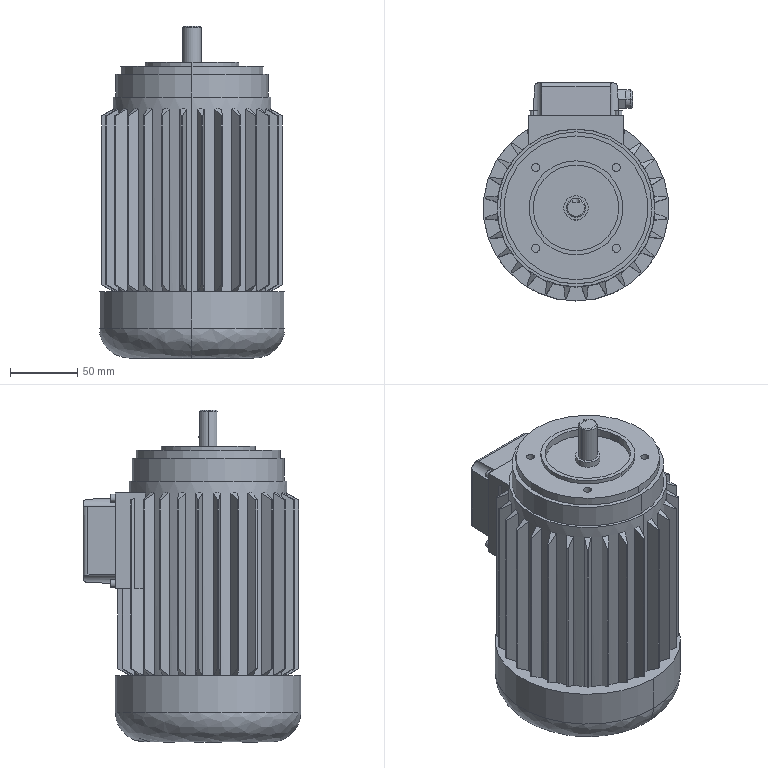Part | STEP file | Motor_P71B14.step | 1 solid | 264 faces | box 138 x 162 x 247 mm | volume 2733778 mm3 | plane 129 | cylinder 76 | cone 55 | spline 4 | commonest cylinder face diameters 135.24 x28 5.763 x8 6 x8 117.3 x7 6.175 x4 12.685 x4